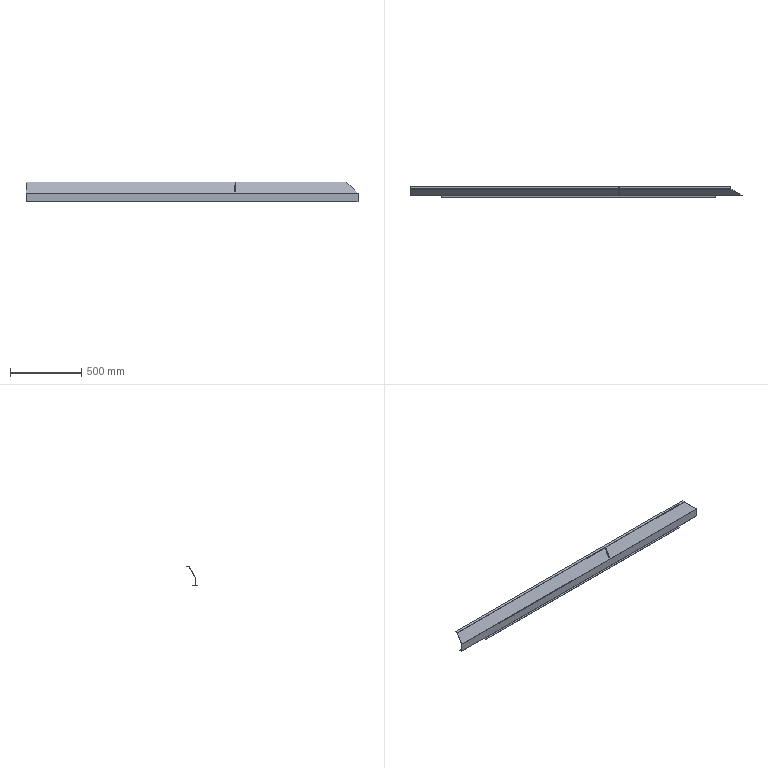Part | STEP file | Front Base Frame | 1 solid | 45 faces | box 2334 x 83.033 x 138 mm | volume 848369 mm3 | plane 31 | cylinder 14 | commonest cylinder face diameters 1 x9 5 x5
STEP:
#1=CARTESIAN_POINT('',(2150.,0.,-56.5));
#2=VERTEX_POINT('',#1);
#3=CARTESIAN_POINT('',(2149.5,0.,-56.));
#4=VERTEX_POINT('',#3);
#5=CARTESIAN_POINT('',(2149.5,0.,-56.5));
#6=DIRECTION('',(0.,-1.,0.));
#7=DIRECTION('',(0.,0.,1.));
#8=AXIS2_PLACEMENT_3D('',#5,#6,#7);
#9=CIRCLE('',#8,0.5);
#10=EDGE_CURVE('',#2,#4,#9,.T.);
#11=ORIENTED_EDGE('',*,*,#10,.T.);
#12=CARTESIAN_POINT('',(2149.5,2.,-56.));
#13=VERTEX_POINT('',#12);
#14=CARTESIAN_POINT('',(2149.5,0.,-56.));
#15=DIRECTION('',(0.,1.,0.));
#16=VECTOR('',#15,1000.);
#17=LINE('',#14,#16);
#18=EDGE_CURVE('',#4,#13,#17,.T.);
#19=ORIENTED_EDGE('',*,*,#18,.T.);
#20=CARTESIAN_POINT('',(2150.,2.,-56.5));
#21=VERTEX_POINT('',#20);
#22=CARTESIAN_POINT('',(2149.5,2.,-56.5));
#23=DIRECTION('',(0.,-1.,0.));
#24=DIRECTION('',(0.,0.,1.));
#25=AXIS2_PLACEMENT_3D('',#22,#23,#24);
#26=CIRCLE('',#25,0.5);
#27=EDGE_CURVE('',#21,#13,#26,.T.);
#28=ORIENTED_EDGE('',*,*,#27,.F.);
#29=CARTESIAN_POINT('',(2150.,0.,-56.5));
#30=DIRECTION('',(0.,1.,0.));
#31=VECTOR('',#30,1000.);
#32=LINE('',#29,#31);
#33=EDGE_CURVE('',#2,#21,#32,.T.);
#34=ORIENTED_EDGE('',*,*,#33,.F.);
#35=EDGE_LOOP('',(#11,#19,#28,#34));
#36=FACE_OUTER_BOUND('',#35,.T.);
#37=CARTESIAN_POINT('',(2149.5,0.,-56.5));
#38=DIRECTION('',(0.,1.,0.));
#39=DIRECTION('',(0.,0.,1.));
#40=AXIS2_PLACEMENT_3D('',#37,#38,#39);
#41=CYLINDRICAL_SURFACE('',#40,0.5);
#42=ADVANCED_FACE('',(#36),#41,.F.);
#43=CARTESIAN_POINT('',(219.5,0.,-56.));
#44=VERTEX_POINT('',#43);
#45=CARTESIAN_POINT('',(220.,0.,-56.5));
#46=VERTEX_POINT('',#45);
#47=CARTESIAN_POINT('',(219.5,0.,-56.5));
#48=DIRECTION('',(0.,1.,0.));
#49=DIRECTION('',(0.,0.,1.));
#50=AXIS2_PLACEMENT_3D('',#47,#48,#49);
#51=CIRCLE('',#50,0.5);
#52=EDGE_CURVE('',#44,#46,#51,.T.);
#53=ORIENTED_EDGE('',*,*,#52,.F.);
#54=CARTESIAN_POINT('',(219.5,2.,-56.));
#55=VERTEX_POINT('',#54);
#56=CARTESIAN_POINT('',(219.5,0.,-56.));
#57=DIRECTION('',(0.,1.,0.));
#58=VECTOR('',#57,1000.);
#59=LINE('',#56,#58);
#60=EDGE_CURVE('',#44,#55,#59,.T.);
#61=ORIENTED_EDGE('',*,*,#60,.T.);
#62=CARTESIAN_POINT('',(220.,2.,-56.5));
#63=VERTEX_POINT('',#62);
#64=CARTESIAN_POINT('',(219.5,2.,-56.5));
#65=DIRECTION('',(0.,-1.,0.));
#66=DIRECTION('',(0.,0.,1.));
#67=AXIS2_PLACEMENT_3D('',#64,#65,#66);
#68=CIRCLE('',#67,0.5);
#69=EDGE_CURVE('',#63,#55,#68,.T.);
#70=ORIENTED_EDGE('',*,*,#69,.F.);
#71=CARTESIAN_POINT('',(220.,0.,-56.5));
#72=DIRECTION('',(0.,1.,0.));
#73=VECTOR('',#72,1000.);
#74=LINE('',#71,#73);
#75=EDGE_CURVE('',#46,#63,#74,.T.);
#76=ORIENTED_EDGE('',*,*,#75,.F.);
#77=EDGE_LOOP('',(#53,#61,#70,#76));
#78=FACE_OUTER_BOUND('',#77,.T.);
#79=CARTESIAN_POINT('',(219.5,0.,-56.5));
#80=DIRECTION('',(0.,1.,0.));
#81=DIRECTION('',(0.,0.,1.));
#82=AXIS2_PLACEMENT_3D('',#79,#80,#81);
#83=CYLINDRICAL_SURFACE('',#82,0.5);
#84=ADVANCED_FACE('',(#78),#83,.F.);
#85=CARTESIAN_POINT('',(0.,2.067,-0.4199));
#86=VERTEX_POINT('',#85);
#87=CARTESIAN_POINT('',(0.,46.044,75.75));
#88=VERTEX_POINT('',#87);
#89=CARTESIAN_POINT('',(0.,46.765,77.));
#90=DIRECTION('',(0.,0.5,0.866));
#91=VECTOR('',#90,1000.);
#92=LINE('',#89,#91);
#93=EDGE_CURVE('',#86,#88,#92,.T.);
#94=ORIENTED_EDGE('',*,*,#93,.T.);
#95=CARTESIAN_POINT('',(1468.,46.044,75.75));
#96=VERTEX_POINT('',#95);
#97=CARTESIAN_POINT('',(2334.,46.044,75.75));
#98=DIRECTION('',(1.,0.,0.));
#99=VECTOR('',#98,1000.);
#100=LINE('',#97,#99);
#101=EDGE_CURVE('',#88,#96,#100,.T.);
#102=ORIENTED_EDGE('',*,*,#101,.T.);
#103=CARTESIAN_POINT('',(1468.,9.238,12.));
#104=VERTEX_POINT('',#103);
#105=CARTESIAN_POINT('',(1468.,46.765,77.));
#106=DIRECTION('',(0.,-0.5,-0.866));
#107=VECTOR('',#106,1000.);
#108=LINE('',#105,#107);
#109=EDGE_CURVE('',#96,#104,#108,.T.);
#110=ORIENTED_EDGE('',*,*,#109,.T.);
#111=CARTESIAN_POINT('',(1473.,9.238,12.));
#112=VERTEX_POINT('',#111);
#113=CARTESIAN_POINT('',(2334.,9.238,12.));
#114=DIRECTION('',(1.,0.,0.));
#115=VECTOR('',#114,1000.);
#116=LINE('',#113,#115);
#117=EDGE_CURVE('',#104,#112,#116,.T.);
#118=ORIENTED_EDGE('',*,*,#117,.T.);
#119=CARTESIAN_POINT('',(1473.,46.044,75.75));
#120=VERTEX_POINT('',#119);
#121=CARTESIAN_POINT('',(1473.,46.765,77.));
#122=DIRECTION('',(0.,0.5,0.866));
#123=VECTOR('',#122,1000.);
#124=LINE('',#121,#123);
#125=EDGE_CURVE('',#112,#120,#124,.T.);
#126=ORIENTED_EDGE('',*,*,#125,.T.);
#127=CARTESIAN_POINT('',(2255.,46.044,75.75));
#128=VERTEX_POINT('',#127);
#129=CARTESIAN_POINT('',(2334.,46.044,75.75));
#130=DIRECTION('',(1.,0.,0.));
#131=VECTOR('',#130,1000.);
#132=LINE('',#129,#131);
#133=EDGE_CURVE('',#120,#128,#132,.T.);
#134=ORIENTED_EDGE('',*,*,#133,.T.);
#135=CARTESIAN_POINT('',(2255.,46.032,75.73));
#136=VERTEX_POINT('',#135);
#137=CARTESIAN_POINT('',(2255.,46.044,75.75));
#138=DIRECTION('',(0.,-0.5,-0.866));
#139=VECTOR('',#138,1000.);
#140=LINE('',#137,#139);
#141=EDGE_CURVE('',#128,#136,#140,.T.);
#142=ORIENTED_EDGE('',*,*,#141,.T.);
#143=CARTESIAN_POINT('',(2333.105,2.067,-0.4199));
#144=VERTEX_POINT('',#143);
#145=CARTESIAN_POINT('',(2255.,46.032,75.73));
#146=DIRECTION('',(0.6641,-0.3738,-0.6475));
#147=VECTOR('',#146,1000.);
#148=LINE('',#145,#147);
#149=EDGE_CURVE('',#136,#144,#148,.T.);
#150=ORIENTED_EDGE('',*,*,#149,.T.);
#151=CARTESIAN_POINT('',(2334.,2.067,-0.4199));
#152=DIRECTION('',(-1.,0.,0.));
#153=VECTOR('',#152,1000.);
#154=LINE('',#151,#153);
#155=EDGE_CURVE('',#144,#86,#154,.T.);
#156=ORIENTED_EDGE('',*,*,#155,.T.);
#157=EDGE_LOOP('',(#94,#102,#110,#118,#126,#134,#142,#150,#156));
#158=FACE_OUTER_BOUND('',#157,.T.);
#159=CARTESIAN_POINT('',(2334.,46.765,77.));
#160=DIRECTION('',(0.,0.866,-0.5));
#161=DIRECTION('',(0.,0.5,0.866));
#162=AXIS2_PLACEMENT_3D('',#159,#160,#161);
#163=PLANE('',#162);
#164=ADVANCED_FACE('',(#158),#163,.T.);
#165=ORIENTED_EDGE('',*,*,#101,.F.);
#166=CARTESIAN_POINT('',(0.,46.477,76.));
#167=VERTEX_POINT('',#166);
#168=CARTESIAN_POINT('',(0.,46.477,75.5));
#169=DIRECTION('',(1.,0.,0.));
#170=DIRECTION('',(0.,0.,1.));
#171=AXIS2_PLACEMENT_3D('',#168,#169,#170);
#172=CIRCLE('',#171,0.5);
#173=EDGE_CURVE('',#167,#88,#172,.T.);
#174=ORIENTED_EDGE('',*,*,#173,.F.);
#175=CARTESIAN_POINT('',(1466.,46.477,76.));
#176=VERTEX_POINT('',#175);
#177=CARTESIAN_POINT('',(2334.,46.477,76.));
#178=DIRECTION('',(-1.,0.,0.));
#179=VECTOR('',#178,1000.);
#180=LINE('',#177,#179);
#181=EDGE_CURVE('',#176,#167,#180,.T.);
#182=ORIENTED_EDGE('',*,*,#181,.F.);
#183=CARTESIAN_POINT('',(1468.,46.477,76.));
#184=VERTEX_POINT('',#183);
#185=CARTESIAN_POINT('',(2334.,46.477,76.));
#186=DIRECTION('',(-1.,0.,0.));
#187=VECTOR('',#186,1000.);
#188=LINE('',#185,#187);
#189=EDGE_CURVE('',#184,#176,#188,.T.);
#190=ORIENTED_EDGE('',*,*,#189,.F.);
#191=CARTESIAN_POINT('',(1468.,46.477,75.5));
#192=DIRECTION('',(-1.,0.,0.));
#193=DIRECTION('',(0.,0.,1.));
#194=AXIS2_PLACEMENT_3D('',#191,#192,#193);
#195=CIRCLE('',#194,0.5);
#196=EDGE_CURVE('',#96,#184,#195,.T.);
#197=ORIENTED_EDGE('',*,*,#196,.F.);
#198=EDGE_LOOP('',(#165,#174,#182,#190,#197));
#199=FACE_OUTER_BOUND('',#198,.T.);
#200=CARTESIAN_POINT('',(2334.,46.477,75.5));
#201=DIRECTION('',(-1.,0.,0.));
#202=DIRECTION('',(0.,0.,1.));
#203=AXIS2_PLACEMENT_3D('',#200,#201,#202);
#204=CYLINDRICAL_SURFACE('',#203,0.5);
#205=ADVANCED_FACE('',(#199),#204,.F.);
#206=ORIENTED_EDGE('',*,*,#93,.F.);
#207=CARTESIAN_POINT('',(0.,2.,-0.6699));
#208=VERTEX_POINT('',#207);
#209=CARTESIAN_POINT('',(0.,2.5,-0.6699));
#210=DIRECTION('',(1.,0.,0.));
#211=DIRECTION('',(0.,0.,1.));
#212=AXIS2_PLACEMENT_3D('',#209,#210,#211);
#213=CIRCLE('',#212,0.5);
#214=EDGE_CURVE('',#86,#208,#213,.T.);
#215=ORIENTED_EDGE('',*,*,#214,.T.);
#216=CARTESIAN_POINT('',(0.,2.,-57.5));
#217=VERTEX_POINT('',#216);
#218=CARTESIAN_POINT('',(0.,2.,0.));
#219=DIRECTION('',(0.,0.,1.));
#220=VECTOR('',#219,1000.);
#221=LINE('',#218,#220);
#222=EDGE_CURVE('',#217,#208,#221,.T.);
#223=ORIENTED_EDGE('',*,*,#222,.F.);
#224=CARTESIAN_POINT('',(0.,2.5,-58.));
#225=VERTEX_POINT('',#224);
#226=CARTESIAN_POINT('',(0.,2.5,-57.5));
#227=DIRECTION('',(1.,0.,0.));
#228=DIRECTION('',(0.,0.,1.));
#229=AXIS2_PLACEMENT_3D('',#226,#227,#228);
#230=CIRCLE('',#229,0.5);
#231=EDGE_CURVE('',#217,#225,#230,.T.);
#232=ORIENTED_EDGE('',*,*,#231,.T.);
#233=CARTESIAN_POINT('',(0.,20.,-58.));
#234=VERTEX_POINT('',#233);
#235=CARTESIAN_POINT('',(0.,0.,-58.));
#236=DIRECTION('',(0.,1.,0.));
#237=VECTOR('',#236,1000.);
#238=LINE('',#235,#237);
#239=EDGE_CURVE('',#225,#234,#238,.T.);
#240=ORIENTED_EDGE('',*,*,#239,.T.);
#241=CARTESIAN_POINT('',(0.,20.,-60.));
#242=VERTEX_POINT('',#241);
#243=CARTESIAN_POINT('',(0.,20.,-60.));
#244=DIRECTION('',(0.,0.,-1.));
#245=VECTOR('',#244,1000.);
#246=LINE('',#243,#245);
#247=EDGE_CURVE('',#234,#242,#246,.T.);
#248=ORIENTED_EDGE('',*,*,#247,.T.);
#249=CARTESIAN_POINT('',(0.,2.5,-60.));
#250=VERTEX_POINT('',#249);
#251=CARTESIAN_POINT('',(0.,2.,-60.));
#252=DIRECTION('',(0.,-1.,0.));
#253=VECTOR('',#252,1000.);
#254=LINE('',#251,#253);
#255=EDGE_CURVE('',#242,#250,#254,.T.);
#256=ORIENTED_EDGE('',*,*,#255,.T.);
#257=CARTESIAN_POINT('',(0.,0.,-57.5));
#258=VERTEX_POINT('',#257);
#259=CARTESIAN_POINT('',(0.,2.5,-57.5));
#260=DIRECTION('',(1.,0.,0.));
#261=DIRECTION('',(0.,0.,1.));
#262=AXIS2_PLACEMENT_3D('',#259,#260,#261);
#263=CIRCLE('',#262,2.5);
#264=EDGE_CURVE('',#258,#250,#263,.T.);
#265=ORIENTED_EDGE('',*,*,#264,.F.);
#266=CARTESIAN_POINT('',(0.,0.,-0.6699));
#267=VERTEX_POINT('',#266);
#268=CARTESIAN_POINT('',(0.,0.,-0.4199));
#269=DIRECTION('',(0.,0.,1.));
#270=VECTOR('',#269,1000.);
#271=LINE('',#268,#270);
#272=EDGE_CURVE('',#258,#267,#271,.T.);
#273=ORIENTED_EDGE('',*,*,#272,.T.);
#274=CARTESIAN_POINT('',(0.,0.3349,0.5801));
#275=VERTEX_POINT('',#274);
#276=CARTESIAN_POINT('',(0.,2.5,-0.6699));
#277=DIRECTION('',(-1.,0.,0.));
#278=DIRECTION('',(0.,0.,1.));
#279=AXIS2_PLACEMENT_3D('',#276,#277,#278);
#280=CIRCLE('',#279,2.5);
#281=EDGE_CURVE('',#267,#275,#280,.T.);
#282=ORIENTED_EDGE('',*,*,#281,.T.);
#283=CARTESIAN_POINT('',(0.,44.312,76.75));
#284=VERTEX_POINT('',#283);
#285=CARTESIAN_POINT('',(0.,0.3349,0.5801));
#286=DIRECTION('',(0.,0.5,0.866));
#287=VECTOR('',#286,1000.);
#288=LINE('',#285,#287);
#289=EDGE_CURVE('',#275,#284,#288,.T.);
#290=ORIENTED_EDGE('',*,*,#289,.T.);
#291=CARTESIAN_POINT('',(0.,46.477,78.));
#292=VERTEX_POINT('',#291);
#293=CARTESIAN_POINT('',(0.,46.477,75.5));
#294=DIRECTION('',(-1.,0.,0.));
#295=DIRECTION('',(0.,0.,1.));
#296=AXIS2_PLACEMENT_3D('',#293,#294,#295);
#297=CIRCLE('',#296,2.5);
#298=EDGE_CURVE('',#284,#292,#297,.T.);
#299=ORIENTED_EDGE('',*,*,#298,.T.);
#300=CARTESIAN_POINT('',(0.,65.033,78.));
#301=VERTEX_POINT('',#300);
#302=CARTESIAN_POINT('',(0.,2.5,78.));
#303=DIRECTION('',(0.,-1.,0.));
#304=VECTOR('',#303,1000.);
#305=LINE('',#302,#304);
#306=EDGE_CURVE('',#301,#292,#305,.T.);
#307=ORIENTED_EDGE('',*,*,#306,.F.);
#308=CARTESIAN_POINT('',(0.,65.033,76.));
#309=VERTEX_POINT('',#308);
#310=CARTESIAN_POINT('',(0.,65.033,78.));
#311=DIRECTION('',(0.,0.,1.));
#312=VECTOR('',#311,1000.);
#313=LINE('',#310,#312);
#314=EDGE_CURVE('',#309,#301,#313,.T.);
#315=ORIENTED_EDGE('',*,*,#314,.F.);
#316=CARTESIAN_POINT('',(0.,65.033,76.));
#317=DIRECTION('',(0.,1.,0.));
#318=VECTOR('',#317,1000.);
#319=LINE('',#316,#318);
#320=EDGE_CURVE('',#167,#309,#319,.T.);
#321=ORIENTED_EDGE('',*,*,#320,.F.);
#322=ORIENTED_EDGE('',*,*,#173,.T.);
#323=EDGE_LOOP('',(#206,#215,#223,#232,#240,#248,#256,#265,#273,#282,#290,#299,#307,#315,#321,#322));
#324=FACE_OUTER_BOUND('',#323,.T.);
#325=CARTESIAN_POINT('',(0.,46.477,76.));
#326=DIRECTION('',(-1.,0.,0.));
#327=DIRECTION('',(0.,0.,1.));
#328=AXIS2_PLACEMENT_3D('',#325,#326,#327);
#329=PLANE('',#328);
#330=ADVANCED_FACE('',(#324),#329,.T.);
#331=CARTESIAN_POINT('',(2333.361,2.,-0.6699));
#332=VERTEX_POINT('',#331);
#333=CARTESIAN_POINT('',(2334.,2.,-0.6699));
#334=DIRECTION('',(1.,0.,0.));
#335=VECTOR('',#334,1000.);
#336=LINE('',#333,#335);
#337=EDGE_CURVE('',#208,#332,#336,.T.);
#338=ORIENTED_EDGE('',*,*,#337,.F.);
#339=ORIENTED_EDGE('',*,*,#214,.F.);
#340=ORIENTED_EDGE('',*,*,#155,.F.);
#341=CARTESIAN_POINT('',(2333.361,2.,-0.6699));
#342=CARTESIAN_POINT('',(2333.271,2.,-0.5816));
#343=CARTESIAN_POINT('',(2333.183,2.023,-0.4963));
#344=CARTESIAN_POINT('',(2333.105,2.067,-0.4199));
#345=(BOUNDED_CURVE()B_SPLINE_CURVE(3,(#341,#342,#343,#344),.UNSPECIFIED.,.F.,.F.)B_SPLINE_CURVE_WITH_KNOTS((4,4),(4.712,5.236),.UNSPECIFIED.)CURVE()GEOMETRIC_REPRESENTATION_ITEM()RATIONAL_B_SPLINE_CURVE((1.,0.9773,0.9773,1.))REPRESENTATION_ITEM(''));
#346=EDGE_CURVE('',#332,#144,#345,.T.);
#347=ORIENTED_EDGE('',*,*,#346,.F.);
#348=EDGE_LOOP('',(#338,#339,#340,#347));
#349=FACE_OUTER_BOUND('',#348,.T.);
#350=CARTESIAN_POINT('',(2334.,2.5,-0.6699));
#351=DIRECTION('',(-1.,0.,0.));
#352=DIRECTION('',(0.,0.,1.));
#353=AXIS2_PLACEMENT_3D('',#350,#351,#352);
#354=CYLINDRICAL_SURFACE('',#353,0.5);
#355=ADVANCED_FACE('',(#349),#354,.F.);
#356=ORIENTED_EDGE('',*,*,#346,.T.);
#357=ORIENTED_EDGE('',*,*,#149,.F.);
#358=CARTESIAN_POINT('',(2255.,43.723,75.73));
#359=VERTEX_POINT('',#358);
#360=CARTESIAN_POINT('',(2255.,-18.,75.73));
#361=DIRECTION('',(0.,1.,0.));
#362=VECTOR('',#361,1000.);
#363=LINE('',#360,#362);
#364=EDGE_CURVE('',#359,#136,#363,.T.);
#365=ORIENTED_EDGE('',*,*,#364,.F.);
#366=CARTESIAN_POINT('',(2332.079,0.3349,0.5801));
#367=VERTEX_POINT('',#366);
#368=CARTESIAN_POINT('',(2332.079,0.3349,0.5801));
#369=DIRECTION('',(-0.6641,0.3738,0.6475));
#370=VECTOR('',#369,1000.);
#371=LINE('',#368,#370);
#372=EDGE_CURVE('',#367,#359,#371,.T.);
#373=ORIENTED_EDGE('',*,*,#372,.F.);
#374=CARTESIAN_POINT('',(2333.361,0.,-0.6699));
#375=VERTEX_POINT('',#374);
#376=CARTESIAN_POINT('',(2333.361,0.,-0.6699));
#377=CARTESIAN_POINT('',(2332.909,0.,-0.2285));
#378=CARTESIAN_POINT('',(2332.471,0.1142,0.1979));
#379=CARTESIAN_POINT('',(2332.079,0.3349,0.5801));
#380=(BOUNDED_CURVE()B_SPLINE_CURVE(3,(#376,#377,#378,#379),.UNSPECIFIED.,.F.,.F.)B_SPLINE_CURVE_WITH_KNOTS((4,4),(4.712,5.236),.UNSPECIFIED.)CURVE()GEOMETRIC_REPRESENTATION_ITEM()RATIONAL_B_SPLINE_CURVE((1.,0.9773,0.9773,1.))REPRESENTATION_ITEM(''));
#381=EDGE_CURVE('',#375,#367,#380,.T.);
#382=ORIENTED_EDGE('',*,*,#381,.F.);
#383=CARTESIAN_POINT('',(2333.7,0.,-1.));
#384=VERTEX_POINT('',#383);
#385=CARTESIAN_POINT('',(2333.361,0.,-0.6699));
#386=DIRECTION('',(0.716,0.,-0.6981));
#387=VECTOR('',#386,1000.);
#388=LINE('',#385,#387);
#389=EDGE_CURVE('',#375,#384,#388,.T.);
#390=ORIENTED_EDGE('',*,*,#389,.T.);
#391=CARTESIAN_POINT('',(2333.7,2.,-1.));
#392=VERTEX_POINT('',#391);
#393=CARTESIAN_POINT('',(2333.7,-18.,-1.));
#394=DIRECTION('',(0.,-1.,0.));
#395=VECTOR('',#394,1000.);
#396=LINE('',#393,#395);
#397=EDGE_CURVE('',#392,#384,#396,.T.);
#398=ORIENTED_EDGE('',*,*,#397,.F.);
#399=CARTESIAN_POINT('',(2255.,2.,75.73));
#400=DIRECTION('',(0.716,0.,-0.6981));
#401=VECTOR('',#400,1000.);
#402=LINE('',#399,#401);
#403=EDGE_CURVE('',#332,#392,#402,.T.);
#404=ORIENTED_EDGE('',*,*,#403,.F.);
#405=EDGE_LOOP('',(#356,#357,#365,#373,#382,#390,#398,#404));
#406=FACE_OUTER_BOUND('',#405,.T.);
#407=CARTESIAN_POINT('',(2255.,-18.,75.73));
#408=DIRECTION('',(-0.6981,0.,-0.716));
#409=DIRECTION('',(-0.716,0.,0.6981));
#410=AXIS2_PLACEMENT_3D('',#407,#408,#409);
#411=PLANE('',#410);
#412=ADVANCED_FACE('',(#406),#411,.F.);
#413=CARTESIAN_POINT('',(2255.,46.477,76.));
#414=VERTEX_POINT('',#413);
#415=CARTESIAN_POINT('',(1473.,46.477,76.));
#416=VERTEX_POINT('',#415);
#417=CARTESIAN_POINT('',(2334.,46.477,76.));
#418=DIRECTION('',(-1.,0.,0.));
#419=VECTOR('',#418,1000.);
#420=LINE('',#417,#419);
#421=EDGE_CURVE('',#414,#416,#420,.T.);
#422=ORIENTED_EDGE('',*,*,#421,.F.);
#423=CARTESIAN_POINT('',(2255.,46.477,75.5));
#424=DIRECTION('',(-1.,0.,0.));
#425=DIRECTION('',(0.,0.,1.));
#426=AXIS2_PLACEMENT_3D('',#423,#424,#425);
#427=CIRCLE('',#426,0.5);
#428=EDGE_CURVE('',#128,#414,#427,.T.);
#429=ORIENTED_EDGE('',*,*,#428,.F.);
#430=ORIENTED_EDGE('',*,*,#133,.F.);
#431=CARTESIAN_POINT('',(1473.,46.477,75.5));
#432=DIRECTION('',(1.,0.,0.));
#433=DIRECTION('',(0.,0.,1.));
#434=AXIS2_PLACEMENT_3D('',#431,#432,#433);
#435=CIRCLE('',#434,0.5);
#436=EDGE_CURVE('',#416,#120,#435,.T.);
#437=ORIENTED_EDGE('',*,*,#436,.F.);
#438=EDGE_LOOP('',(#422,#429,#430,#437));
#439=FACE_OUTER_BOUND('',#438,.T.);
#440=CARTESIAN_POINT('',(2334.,46.477,75.5));
#441=DIRECTION('',(-1.,0.,0.));
#442=DIRECTION('',(0.,0.,1.));
#443=AXIS2_PLACEMENT_3D('',#440,#441,#442);
#444=CYLINDRICAL_SURFACE('',#443,0.5);
#445=ADVANCED_FACE('',(#439),#444,.F.);
#446=ORIENTED_EDGE('',*,*,#436,.T.);
#447=ORIENTED_EDGE('',*,*,#125,.F.);
#448=CARTESIAN_POINT('',(1473.,6.928,12.));
#449=VERTEX_POINT('',#448);
#450=CARTESIAN_POINT('',(1473.,-18.,12.));
#451=DIRECTION('',(0.,1.,0.));
#452=VECTOR('',#451,1000.);
#453=LINE('',#450,#452);
#454=EDGE_CURVE('',#449,#112,#453,.T.);
#455=ORIENTED_EDGE('',*,*,#454,.F.);
#456=CARTESIAN_POINT('',(1473.,44.312,76.75));
#457=VERTEX_POINT('',#456);
#458=CARTESIAN_POINT('',(1473.,44.312,76.75));
#459=DIRECTION('',(0.,-0.5,-0.866));
#460=VECTOR('',#459,1000.);
#461=LINE('',#458,#460);
#462=EDGE_CURVE('',#457,#449,#461,.T.);
#463=ORIENTED_EDGE('',*,*,#462,.F.);
#464=CARTESIAN_POINT('',(1473.,46.477,78.));
#465=VERTEX_POINT('',#464);
#466=CARTESIAN_POINT('',(1473.,46.477,75.5));
#467=DIRECTION('',(1.,0.,0.));
#468=DIRECTION('',(0.,0.,1.));
#469=AXIS2_PLACEMENT_3D('',#466,#467,#468);
#470=CIRCLE('',#469,2.5);
#471=EDGE_CURVE('',#465,#457,#470,.T.);
#472=ORIENTED_EDGE('',*,*,#471,.F.);
#473=CARTESIAN_POINT('',(1473.,65.033,78.));
#474=VERTEX_POINT('',#473);
#475=CARTESIAN_POINT('',(1473.,-18.,78.));
#476=DIRECTION('',(0.,-1.,0.));
#477=VECTOR('',#476,1000.);
#478=LINE('',#475,#477);
#479=EDGE_CURVE('',#474,#465,#478,.T.);
#480=ORIENTED_EDGE('',*,*,#479,.F.);
#481=CARTESIAN_POINT('',(1473.,65.033,76.));
#482=VERTEX_POINT('',#481);
#483=CARTESIAN_POINT('',(1473.,65.033,78.));
#484=DIRECTION('',(0.,0.,1.));
#485=VECTOR('',#484,1000.);
#486=LINE('',#483,#485);
#487=EDGE_CURVE('',#482,#474,#486,.T.);
#488=ORIENTED_EDGE('',*,*,#487,.F.);
#489=CARTESIAN_POINT('',(1473.,-18.,76.));
#490=DIRECTION('',(0.,1.,0.));
#491=VECTOR('',#490,1000.);
#492=LINE('',#489,#491);
#493=EDGE_CURVE('',#416,#482,#492,.T.);
#494=ORIENTED_EDGE('',*,*,#493,.F.);
#495=EDGE_LOOP('',(#446,#447,#455,#463,#472,#480,#488,#494));
#496=FACE_OUTER_BOUND('',#495,.T.);
#497=CARTESIAN_POINT('',(1473.,-18.,78.));
#498=DIRECTION('',(1.,0.,0.));
#499=DIRECTION('',(0.,0.,-1.));
#500=AXIS2_PLACEMENT_3D('',#497,#498,#499);
#501=PLANE('',#500);
#502=ADVANCED_FACE('',(#496),#501,.F.);
#503=CARTESIAN_POINT('',(1468.,6.928,12.));
#504=VERTEX_POINT('',#503);
#505=CARTESIAN_POINT('',(1468.,-18.,12.));
#506=DIRECTION('',(0.,1.,0.));
#507=VECTOR('',#506,1000.);
#508=LINE('',#505,#507);
#509=EDGE_CURVE('',#504,#104,#508,.T.);
#510=ORIENTED_EDGE('',*,*,#509,.F.);
#511=CARTESIAN_POINT('',(1468.,6.928,12.));
#512=DIRECTION('',(-1.,0.,0.));
#513=VECTOR('',#512,1000.);
#514=LINE('',#511,#513);
#515=EDGE_CURVE('',#449,#504,#514,.T.);
#516=ORIENTED_EDGE('',*,*,#515,.F.);
#517=ORIENTED_EDGE('',*,*,#454,.T.);
#518=ORIENTED_EDGE('',*,*,#117,.F.);
#519=EDGE_LOOP('',(#510,#516,#517,#518));
#520=FACE_OUTER_BOUND('',#519,.T.);
#521=CARTESIAN_POINT('',(1468.,-18.,12.));
#522=DIRECTION('',(0.,0.,-1.));
#523=DIRECTION('',(0.,1.,0.));
#524=AXIS2_PLACEMENT_3D('',#521,#522,#523);
#525=PLANE('',#524);
#526=ADVANCED_FACE('',(#520),#525,.F.);
#527=ORIENTED_EDGE('',*,*,#109,.F.);
#528=ORIENTED_EDGE('',*,*,#196,.T.);
#529=CARTESIAN_POINT('',(1468.,46.477,78.));
#530=VERTEX_POINT('',#529);
#531=CARTESIAN_POINT('',(1468.,46.477,78.));
#532=DIRECTION('',(0.,0.,-1.));
#533=VECTOR('',#532,1000.);
#534=LINE('',#531,#533);
#535=EDGE_CURVE('',#530,#184,#534,.T.);
#536=ORIENTED_EDGE('',*,*,#535,.F.);
#537=CARTESIAN_POINT('',(1468.,44.312,76.75));
#538=VERTEX_POINT('',#537);
#539=CARTESIAN_POINT('',(1468.,46.477,75.5));
#540=DIRECTION('',(-1.,0.,0.));
#541=DIRECTION('',(0.,0.,1.));
#542=AXIS2_PLACEMENT_3D('',#539,#540,#541);
#543=CIRCLE('',#542,2.5);
#544=EDGE_CURVE('',#538,#530,#543,.T.);
#545=ORIENTED_EDGE('',*,*,#544,.F.);
#546=CARTESIAN_POINT('',(1468.,6.928,12.));
#547=DIRECTION('',(0.,0.5,0.866));
#548=VECTOR('',#547,1000.);
#549=LINE('',#546,#548);
#550=EDGE_CURVE('',#504,#538,#549,.T.);
#551=ORIENTED_EDGE('',*,*,#550,.F.);
#552=ORIENTED_EDGE('',*,*,#509,.T.);
#553=EDGE_LOOP('',(#527,#528,#536,#545,#551,#552));
#554=FACE_OUTER_BOUND('',#553,.T.);
#555=CARTESIAN_POINT('',(1468.,-18.,78.));
#556=DIRECTION('',(-1.,0.,0.));
#557=DIRECTION('',(0.,0.,1.));
#558=AXIS2_PLACEMENT_3D('',#555,#556,#557);
#559=PLANE('',#558);
#560=ADVANCED_FACE('',(#554),#559,.F.);
#561=ORIENTED_EDGE('',*,*,#320,.T.);
#562=CARTESIAN_POINT('',(1466.,65.033,76.));
#563=VERTEX_POINT('',#562);
#564=CARTESIAN_POINT('',(2334.,65.033,76.));
#565=DIRECTION('',(1.,0.,0.));
#566=VECTOR('',#565,1000.);
#567=LINE('',#564,#566);
#568=EDGE_CURVE('',#309,#563,#567,.T.);
#569=ORIENTED_EDGE('',*,*,#568,.T.);
#570=CARTESIAN_POINT('',(1466.,65.033,76.));
#571=DIRECTION('',(0.,-1.,0.));
#572=VECTOR('',#571,1000.);
#573=LINE('',#570,#572);
#574=EDGE_CURVE('',#563,#176,#573,.T.);
#575=ORIENTED_EDGE('',*,*,#574,.T.);
#576=ORIENTED_EDGE('',*,*,#181,.T.);
#577=EDGE_LOOP('',(#561,#569,#575,#576));
#578=FACE_OUTER_BOUND('',#577,.T.);
#579=CARTESIAN_POINT('',(2334.,65.033,76.));
#580=DIRECTION('',(0.,0.,-1.));
#581=DIRECTION('',(0.,1.,0.));
#582=AXIS2_PLACEMENT_3D('',#579,#580,#581);
#583=PLANE('',#582);
#584=ADVANCED_FACE('',(#578),#583,.T.);
#585=ORIENTED_EDGE('',*,*,#535,.T.);
#586=ORIENTED_EDGE('',*,*,#189,.T.);
#587=CARTESIAN_POINT('',(1466.,46.477,78.));
#588=VERTEX_POINT('',#587);
#589=CARTESIAN_POINT('',(1466.,46.477,78.));
#590=DIRECTION('',(0.,0.,-1.));
#591=VECTOR('',#590,1000.);
#592=LINE('',#589,#591);
#593=EDGE_CURVE('',#588,#176,#592,.T.);
#594=ORIENTED_EDGE('',*,*,#593,.F.);
#595=CARTESIAN_POINT('',(1472.,46.477,78.));
#596=DIRECTION('',(-1.,0.,0.));
#597=VECTOR('',#596,1000.);
#598=LINE('',#595,#597);
#599=EDGE_CURVE('',#530,#588,#598,.T.);
#600=ORIENTED_EDGE('',*,*,#599,.F.);
#601=EDGE_LOOP('',(#585,#586,#594,#600));
#602=FACE_OUTER_BOUND('',#601,.T.);
#603=CARTESIAN_POINT('',(1472.,46.477,78.));
#604=DIRECTION('',(0.,-1.,0.));
#605=DIRECTION('',(0.,0.,-1.));
#606=AXIS2_PLACEMENT_3D('',#603,#604,#605);
#607=PLANE('',#606);
#608=ADVANCED_FACE('',(#602),#607,.F.);
#609=ORIENTED_EDGE('',*,*,#550,.T.);
#610=CARTESIAN_POINT('',(2334.,44.312,76.75));
#611=DIRECTION('',(1.,0.,0.));
#612=VECTOR('',#611,1000.);
#613=LINE('',#610,#612);
#614=EDGE_CURVE('',#284,#538,#613,.T.);
#615=ORIENTED_EDGE('',*,*,#614,.F.);
#616=ORIENTED_EDGE('',*,*,#289,.F.);
#617=CARTESIAN_POINT('',(2334.,0.3349,0.5801));
#618=DIRECTION('',(-1.,0.,0.));
#619=VECTOR('',#618,1000.);
#620=LINE('',#617,#619);
#621=EDGE_CURVE('',#367,#275,#620,.T.);
#622=ORIENTED_EDGE('',*,*,#621,.F.);
#623=ORIENTED_EDGE('',*,*,#372,.T.);
#624=CARTESIAN_POINT('',(2255.,44.312,76.75));
#625=VERTEX_POINT('',#624);
#626=CARTESIAN_POINT('',(2255.,45.033,78.));
#627=DIRECTION('',(0.,-0.5,-0.866));
#628=VECTOR('',#627,1000.);
#629=LINE('',#626,#628);
#630=EDGE_CURVE('',#625,#359,#629,.T.);
#631=ORIENTED_EDGE('',*,*,#630,.F.);
#632=CARTESIAN_POINT('',(2334.,44.312,76.75));
#633=DIRECTION('',(1.,0.,0.));
#634=VECTOR('',#633,1000.);
#635=LINE('',#632,#634);
#636=EDGE_CURVE('',#457,#625,#635,.T.);
#637=ORIENTED_EDGE('',*,*,#636,.F.);
#638=ORIENTED_EDGE('',*,*,#462,.T.);
#639=ORIENTED_EDGE('',*,*,#515,.T.);
#640=EDGE_LOOP('',(#609,#615,#616,#622,#623,#631,#637,#638,#639));
#641=FACE_OUTER_BOUND('',#640,.T.);
#642=CARTESIAN_POINT('',(2334.,45.033,78.));
#643=DIRECTION('',(0.,0.866,-0.5));
#644=DIRECTION('',(0.,0.5,0.866));
#645=AXIS2_PLACEMENT_3D('',#642,#643,#644);
#646=PLANE('',#645);
#647=ADVANCED_FACE('',(#641),#646,.F.);
#648=ORIENTED_EDGE('',*,*,#222,.T.);
#649=ORIENTED_EDGE('',*,*,#337,.T.);
#650=ORIENTED_EDGE('',*,*,#403,.T.);
#651=CARTESIAN_POINT('',(2334.,2.,-1.));
#652=VERTEX_POINT('',#651);
#653=CARTESIAN_POINT('',(2334.,2.,-1.));
#654=DIRECTION('',(1.,0.,0.));
#655=VECTOR('',#654,1000.);
#656=LINE('',#653,#655);
#657=EDGE_CURVE('',#392,#652,#656,.T.);
#658=ORIENTED_EDGE('',*,*,#657,.T.);
#659=CARTESIAN_POINT('',(2334.,2.,-60.));
#660=VERTEX_POINT('',#659);
#661=CARTESIAN_POINT('',(2334.,2.,0.));
#662=DIRECTION('',(0.,0.,-1.));
#663=VECTOR('',#662,1000.);
#664=LINE('',#661,#663);
#665=EDGE_CURVE('',#652,#660,#664,.T.);
#666=ORIENTED_EDGE('',*,*,#665,.T.);
#667=CARTESIAN_POINT('',(2150.,2.,-60.));
#668=VERTEX_POINT('',#667);
#669=CARTESIAN_POINT('',(2334.,2.,-60.));
#670=DIRECTION('',(-1.,0.,0.));
#671=VECTOR('',#670,1000.);
#672=LINE('',#669,#671);
#673=EDGE_CURVE('',#660,#668,#672,.T.);
#674=ORIENTED_EDGE('',*,*,#673,.T.);
#675=CARTESIAN_POINT('',(2150.,2.,0.));
#676=DIRECTION('',(0.,0.,1.));
#677=VECTOR('',#676,1000.);
#678=LINE('',#675,#677);
#679=EDGE_CURVE('',#668,#21,#678,.T.);
#680=ORIENTED_EDGE('',*,*,#679,.T.);
#681=ORIENTED_EDGE('',*,*,#27,.T.);
#682=CARTESIAN_POINT('',(2149.,2.,-56.5));
#683=VERTEX_POINT('',#682);
#684=CARTESIAN_POINT('',(2149.5,2.,-56.5));
#685=DIRECTION('',(0.,-1.,0.));
#686=DIRECTION('',(0.,0.,1.));
#687=AXIS2_PLACEMENT_3D('',#684,#685,#686);
#688=CIRCLE('',#687,0.5);
#689=EDGE_CURVE('',#13,#683,#688,.T.);
#690=ORIENTED_EDGE('',*,*,#689,.T.);
#691=CARTESIAN_POINT('',(2149.,2.,-57.5));
#692=VERTEX_POINT('',#691);
#693=CARTESIAN_POINT('',(2149.,2.,-56.5));
#694=DIRECTION('',(0.,0.,1.));
#695=VECTOR('',#694,1000.);
#696=LINE('',#693,#695);
#697=EDGE_CURVE('',#692,#683,#696,.T.);
#698=ORIENTED_EDGE('',*,*,#697,.F.);
#699=CARTESIAN_POINT('',(220.,2.,-57.5));
#700=VERTEX_POINT('',#699);
#701=CARTESIAN_POINT('',(2334.,2.,-57.5));
#702=DIRECTION('',(-1.,0.,0.));
#703=VECTOR('',#702,1000.);
#704=LINE('',#701,#703);
#705=EDGE_CURVE('',#692,#700,#704,.T.);
#706=ORIENTED_EDGE('',*,*,#705,.T.);
#707=CARTESIAN_POINT('',(220.,2.,-57.5));
#708=DIRECTION('',(0.,0.,-1.));
#709=VECTOR('',#708,1000.);
#710=LINE('',#707,#709);
#711=EDGE_CURVE('',#63,#700,#710,.T.);
#712=ORIENTED_EDGE('',*,*,#711,.F.);
#713=ORIENTED_EDGE('',*,*,#69,.T.);
#714=CARTESIAN_POINT('',(219.,2.,-56.5));
#715=VERTEX_POINT('',#714);
#716=CARTESIAN_POINT('',(219.5,2.,-56.5));
#717=DIRECTION('',(0.,-1.,0.));
#718=DIRECTION('',(0.,0.,1.));
#719=AXIS2_PLACEMENT_3D('',#716,#717,#718);
#720=CIRCLE('',#719,0.5);
#721=EDGE_CURVE('',#55,#715,#720,.T.);
#722=ORIENTED_EDGE('',*,*,#721,.T.);
#723=CARTESIAN_POINT('',(219.,2.,-57.5));
#724=VERTEX_POINT('',#723);
#725=CARTESIAN_POINT('',(219.,2.,-56.5));
#726=DIRECTION('',(0.,0.,1.));
#727=VECTOR('',#726,1000.);
#728=LINE('',#725,#727);
#729=EDGE_CURVE('',#724,#715,#728,.T.);
#730=ORIENTED_EDGE('',*,*,#729,.F.);
#731=CARTESIAN_POINT('',(2334.,2.,-57.5));
#732=DIRECTION('',(-1.,0.,0.));
#733=VECTOR('',#732,1000.);
#734=LINE('',#731,#733);
#735=EDGE_CURVE('',#724,#217,#734,.T.);
#736=ORIENTED_EDGE('',*,*,#735,.T.);
#737=EDGE_LOOP('',(#648,#649,#650,#658,#666,#674,#680,#681,#690,#698,#706,#712,#713,#722,#730,#736));
#738=FACE_OUTER_BOUND('',#737,.T.);
#739=CARTESIAN_POINT('',(2334.,2.,0.));
#740=DIRECTION('',(0.,1.,0.));
#741=DIRECTION('',(0.,0.,1.));
#742=AXIS2_PLACEMENT_3D('',#739,#740,#741);
#743=PLANE('',#742);
#744=ADVANCED_FACE('',(#738),#743,.T.);
#745=ORIENTED_EDGE('',*,*,#428,.T.);
#746=CARTESIAN_POINT('',(2255.,65.033,76.));
#747=VERTEX_POINT('',#746);
#748=CARTESIAN_POINT('',(2255.,-18.,76.));
#749=DIRECTION('',(0.,-1.,0.));
#750=VECTOR('',#749,1000.);
#751=LINE('',#748,#750);
#752=EDGE_CURVE('',#747,#414,#751,.T.);
#753=ORIENTED_EDGE('',*,*,#752,.F.);
#754=CARTESIAN_POINT('',(2255.,65.033,78.));
#755=VERTEX_POINT('',#754);
#756=CARTESIAN_POINT('',(2255.,65.033,75.73));
#757=DIRECTION('',(0.,0.,-1.));
#758=VECTOR('',#757,1000.);
#759=LINE('',#756,#758);
#760=EDGE_CURVE('',#755,#747,#759,.T.);
#761=ORIENTED_EDGE('',*,*,#760,.F.);
#762=CARTESIAN_POINT('',(2255.,46.477,78.));
#763=VERTEX_POINT('',#762);
#764=CARTESIAN_POINT('',(2255.,-18.,78.));
#765=DIRECTION('',(0.,1.,0.));
#766=VECTOR('',#765,1000.);
#767=LINE('',#764,#766);
#768=EDGE_CURVE('',#763,#755,#767,.T.);
#769=ORIENTED_EDGE('',*,*,#768,.F.);
#770=CARTESIAN_POINT('',(2255.,46.477,75.5));
#771=DIRECTION('',(-1.,0.,0.));
#772=DIRECTION('',(0.,0.,1.));
#773=AXIS2_PLACEMENT_3D('',#770,#771,#772);
#774=CIRCLE('',#773,2.5);
#775=EDGE_CURVE('',#625,#763,#774,.T.);
#776=ORIENTED_EDGE('',*,*,#775,.F.);
#777=ORIENTED_EDGE('',*,*,#630,.T.);
#778=ORIENTED_EDGE('',*,*,#364,.T.);
#779=ORIENTED_EDGE('',*,*,#141,.F.);
#780=EDGE_LOOP('',(#745,#753,#761,#769,#776,#777,#778,#779));
#781=FACE_OUTER_BOUND('',#780,.T.);
#782=CARTESIAN_POINT('',(2255.,-18.,75.73));
#783=DIRECTION('',(-1.,0.,0.));
#784=DIRECTION('',(0.,0.,1.));
#785=AXIS2_PLACEMENT_3D('',#782,#783,#784);
#786=PLANE('',#785);
#787=ADVANCED_FACE('',(#781),#786,.F.);
#788=ORIENTED_EDGE('',*,*,#621,.T.);
#789=ORIENTED_EDGE('',*,*,#281,.F.);
#790=CARTESIAN_POINT('',(2334.,0.,-0.6699));
#791=DIRECTION('',(1.,0.,0.));
#792=VECTOR('',#791,1000.);
#793=LINE('',#790,#792);
#794=EDGE_CURVE('',#267,#375,#793,.T.);
#795=ORIENTED_EDGE('',*,*,#794,.T.);
#796=ORIENTED_EDGE('',*,*,#381,.T.);
#797=EDGE_LOOP('',(#788,#789,#795,#796));
#798=FACE_OUTER_BOUND('',#797,.T.);
#799=CARTESIAN_POINT('',(2334.,2.5,-0.6699));
#800=DIRECTION('',(-1.,0.,0.));
#801=DIRECTION('',(0.,0.,1.));
#802=AXIS2_PLACEMENT_3D('',#799,#800,#801);
#803=CYLINDRICAL_SURFACE('',#802,2.5);
#804=ADVANCED_FACE('',(#798),#803,.T.);
#805=ORIENTED_EDGE('',*,*,#657,.F.);
#806=ORIENTED_EDGE('',*,*,#397,.T.);
#807=CARTESIAN_POINT('',(2334.,0.,-1.));
#808=VERTEX_POINT('',#807);
#809=CARTESIAN_POINT('',(2334.,0.,-1.));
#810=DIRECTION('',(-1.,0.,0.));
#811=VECTOR('',#810,1000.);
#812=LINE('',#809,#811);
#813=EDGE_CURVE('',#808,#384,#812,.T.);
#814=ORIENTED_EDGE('',*,*,#813,.F.);
#815=CARTESIAN_POINT('',(2334.,-18.,-1.));
#816=DIRECTION('',(0.,-1.,0.));
#817=VECTOR('',#816,1000.);
#818=LINE('',#815,#817);
#819=EDGE_CURVE('',#652,#808,#818,.T.);
#820=ORIENTED_EDGE('',*,*,#819,.F.);
#821=EDGE_LOOP('',(#805,#806,#814,#820));
#822=FACE_OUTER_BOUND('',#821,.T.);
#823=CARTESIAN_POINT('',(2334.,-18.,-1.));
#824=DIRECTION('',(0.,0.,-1.));
#825=DIRECTION('',(0.,1.,0.));
#826=AXIS2_PLACEMENT_3D('',#823,#824,#825);
#827=PLANE('',#826);
#828=ADVANCED_FACE('',(#822),#827,.F.);
#829=ORIENTED_EDGE('',*,*,#752,.T.);
#830=ORIENTED_EDGE('',*,*,#421,.T.);
#831=ORIENTED_EDGE('',*,*,#493,.T.);
#832=CARTESIAN_POINT('',(2334.,65.033,76.));
#833=DIRECTION('',(1.,0.,0.));
#834=VECTOR('',#833,1000.);
#835=LINE('',#832,#834);
#836=EDGE_CURVE('',#482,#747,#835,.T.);
#837=ORIENTED_EDGE('',*,*,#836,.T.);
#838=EDGE_LOOP('',(#829,#830,#831,#837));
#839=FACE_OUTER_BOUND('',#838,.T.);
#840=CARTESIAN_POINT('',(2334.,65.033,76.));
#841=DIRECTION('',(0.,0.,-1.));
#842=DIRECTION('',(0.,1.,0.));
#843=AXIS2_PLACEMENT_3D('',#840,#841,#842);
#844=PLANE('',#843);
#845=ADVANCED_FACE('',(#839),#844,.T.);
#846=ORIENTED_EDGE('',*,*,#636,.T.);
#847=ORIENTED_EDGE('',*,*,#775,.T.);
#848=CARTESIAN_POINT('',(2334.,46.477,78.));
#849=DIRECTION('',(-1.,0.,0.));
#850=VECTOR('',#849,1000.);
#851=LINE('',#848,#850);
#852=EDGE_CURVE('',#763,#465,#851,.T.);
#853=ORIENTED_EDGE('',*,*,#852,.T.);
#854=ORIENTED_EDGE('',*,*,#471,.T.);
#855=EDGE_LOOP('',(#846,#847,#853,#854));
#856=FACE_OUTER_BOUND('',#855,.T.);
#857=CARTESIAN_POINT('',(2334.,46.477,75.5));
#858=DIRECTION('',(-1.,0.,0.));
#859=DIRECTION('',(0.,0.,1.));
#860=AXIS2_PLACEMENT_3D('',#857,#858,#859);
#861=CYLINDRICAL_SURFACE('',#860,2.5);
#862=ADVANCED_FACE('',(#856),#861,.T.);
#863=ORIENTED_EDGE('',*,*,#479,.T.);
#864=ORIENTED_EDGE('',*,*,#852,.F.);
#865=ORIENTED_EDGE('',*,*,#768,.T.);
#866=CARTESIAN_POINT('',(2334.,65.033,78.));
#867=DIRECTION('',(1.,0.,0.));
#868=VECTOR('',#867,1000.);
#869=LINE('',#866,#868);
#870=EDGE_CURVE('',#474,#755,#869,.T.);
#871=ORIENTED_EDGE('',*,*,#870,.F.);
#872=EDGE_LOOP('',(#863,#864,#865,#871));
#873=FACE_OUTER_BOUND('',#872,.T.);
#874=CARTESIAN_POINT('',(2334.,65.033,78.));
#875=DIRECTION('',(0.,0.,-1.));
#876=DIRECTION('',(0.,1.,0.));
#877=AXIS2_PLACEMENT_3D('',#874,#875,#876);
#878=PLANE('',#877);
#879=ADVANCED_FACE('',(#873),#878,.F.);
#880=ORIENTED_EDGE('',*,*,#760,.T.);
#881=ORIENTED_EDGE('',*,*,#836,.F.);
#882=ORIENTED_EDGE('',*,*,#487,.T.);
#883=ORIENTED_EDGE('',*,*,#870,.T.);
#884=EDGE_LOOP('',(#880,#881,#882,#883));
#885=FACE_OUTER_BOUND('',#884,.T.);
#886=CARTESIAN_POINT('',(2334.,65.033,78.));
#887=DIRECTION('',(0.,1.,0.));
#888=DIRECTION('',(0.,0.,1.));
#889=AXIS2_PLACEMENT_3D('',#886,#887,#888);
#890=PLANE('',#889);
#891=ADVANCED_FACE('',(#885),#890,.T.);
#892=CARTESIAN_POINT('',(2334.,46.477,78.));
#893=DIRECTION('',(-1.,0.,0.));
#894=VECTOR('',#893,1000.);
#895=LINE('',#892,#894);
#896=EDGE_CURVE('',#588,#292,#895,.T.);
#897=ORIENTED_EDGE('',*,*,#896,.T.);
#898=ORIENTED_EDGE('',*,*,#298,.F.);
#899=ORIENTED_EDGE('',*,*,#614,.T.);
#900=ORIENTED_EDGE('',*,*,#544,.T.);
#901=ORIENTED_EDGE('',*,*,#599,.T.);
#902=EDGE_LOOP('',(#897,#898,#899,#900,#901));
#903=FACE_OUTER_BOUND('',#902,.T.);
#904=CARTESIAN_POINT('',(2334.,46.477,75.5));
#905=DIRECTION('',(-1.,0.,0.));
#906=DIRECTION('',(0.,0.,1.));
#907=AXIS2_PLACEMENT_3D('',#904,#905,#906);
#908=CYLINDRICAL_SURFACE('',#907,2.5);
#909=ADVANCED_FACE('',(#903),#908,.T.);
#910=ORIENTED_EDGE('',*,*,#314,.T.);
#911=CARTESIAN_POINT('',(1466.,65.033,78.));
#912=VERTEX_POINT('',#911);
#913=CARTESIAN_POINT('',(2334.,65.033,78.));
#914=DIRECTION('',(1.,0.,0.));
#915=VECTOR('',#914,1000.);
#916=LINE('',#913,#915);
#917=EDGE_CURVE('',#301,#912,#916,.T.);
#918=ORIENTED_EDGE('',*,*,#917,.T.);
#919=CARTESIAN_POINT('',(1466.,65.033,78.));
#920=DIRECTION('',(0.,0.,-1.));
#921=VECTOR('',#920,1000.);
#922=LINE('',#919,#921);
#923=EDGE_CURVE('',#912,#563,#922,.T.);
#924=ORIENTED_EDGE('',*,*,#923,.T.);
#925=ORIENTED_EDGE('',*,*,#568,.F.);
#926=EDGE_LOOP('',(#910,#918,#924,#925));
#927=FACE_OUTER_BOUND('',#926,.T.);
#928=CARTESIAN_POINT('',(2334.,65.033,78.));
#929=DIRECTION('',(0.,1.,0.));
#930=DIRECTION('',(0.,0.,1.));
#931=AXIS2_PLACEMENT_3D('',#928,#929,#930);
#932=PLANE('',#931);
#933=ADVANCED_FACE('',(#927),#932,.T.);
#934=ORIENTED_EDGE('',*,*,#923,.F.);
#935=CARTESIAN_POINT('',(1466.,65.033,78.));
#936=DIRECTION('',(0.,1.,0.));
#937=VECTOR('',#936,1000.);
#938=LINE('',#935,#937);
#939=EDGE_CURVE('',#588,#912,#938,.T.);
#940=ORIENTED_EDGE('',*,*,#939,.F.);
#941=ORIENTED_EDGE('',*,*,#593,.T.);
#942=ORIENTED_EDGE('',*,*,#574,.F.);
#943=EDGE_LOOP('',(#934,#940,#941,#942));
#944=FACE_OUTER_BOUND('',#943,.T.);
#945=CARTESIAN_POINT('',(1466.,65.033,78.));
#946=DIRECTION('',(-1.,0.,0.));
#947=DIRECTION('',(0.,0.,1.));
#948=AXIS2_PLACEMENT_3D('',#945,#946,#947);
#949=PLANE('',#948);
#950=ADVANCED_FACE('',(#944),#949,.F.);
#951=CARTESIAN_POINT('',(219.,2.5,-58.));
#952=VERTEX_POINT('',#951);
#953=CARTESIAN_POINT('',(219.,2.5,-57.5));
#954=DIRECTION('',(-1.,0.,0.));
#955=DIRECTION('',(0.,0.,1.));
#956=AXIS2_PLACEMENT_3D('',#953,#954,#955);
#957=CIRCLE('',#956,0.5);
#958=EDGE_CURVE('',#952,#724,#957,.T.);
#959=ORIENTED_EDGE('',*,*,#958,.F.);
#960=CARTESIAN_POINT('',(0.,2.5,-58.));
#961=DIRECTION('',(1.,0.,0.));
#962=VECTOR('',#961,1000.);
#963=LINE('',#960,#962);
#964=EDGE_CURVE('',#225,#952,#963,.T.);
#965=ORIENTED_EDGE('',*,*,#964,.F.);
#966=ORIENTED_EDGE('',*,*,#231,.F.);
#967=ORIENTED_EDGE('',*,*,#735,.F.);
#968=EDGE_LOOP('',(#959,#965,#966,#967));
#969=FACE_OUTER_BOUND('',#968,.T.);
#970=CARTESIAN_POINT('',(0.,2.5,-57.5));
#971=DIRECTION('',(-1.,0.,0.));
#972=DIRECTION('',(0.,0.,1.));
#973=AXIS2_PLACEMENT_3D('',#970,#971,#972);
#974=CYLINDRICAL_SURFACE('',#973,0.5);
#975=ADVANCED_FACE('',(#969),#974,.F.);
#976=CARTESIAN_POINT('',(2149.,-0.5,-60.));
#977=VERTEX_POINT('',#976);
#978=CARTESIAN_POINT('',(220.,-0.5,-60.));
#979=VERTEX_POINT('',#978);
#980=CARTESIAN_POINT('',(2149.,-0.5,-60.));
#981=DIRECTION('',(-1.,0.,0.));
#982=VECTOR('',#981,1000.);
#983=LINE('',#980,#982);
#984=EDGE_CURVE('',#977,#979,#983,.T.);
#985=ORIENTED_EDGE('',*,*,#984,.T.);
#986=CARTESIAN_POINT('',(220.,-0.5,-57.5));
#987=DIRECTION('',(1.,0.,0.));
#988=DIRECTION('',(0.,1.,0.));
#989=AXIS2_PLACEMENT_3D('',#986,#987,#988);
#990=CIRCLE('',#989,2.5);
#991=EDGE_CURVE('',#979,#700,#990,.T.);
#992=ORIENTED_EDGE('',*,*,#991,.T.);
#993=ORIENTED_EDGE('',*,*,#705,.F.);
#994=CARTESIAN_POINT('',(2149.,-0.5,-57.5));
#995=DIRECTION('',(-1.,0.,0.));
#996=DIRECTION('',(0.,1.,0.));
#997=AXIS2_PLACEMENT_3D('',#994,#995,#996);
#998=CIRCLE('',#997,2.5);
#999=EDGE_CURVE('',#692,#977,#998,.T.);
#1000=ORIENTED_EDGE('',*,*,#999,.T.);
#1001=EDGE_LOOP('',(#985,#992,#993,#1000));
#1002=FACE_OUTER_BOUND('',#1001,.T.);
#1003=CARTESIAN_POINT('',(2149.,-0.5,-57.5));
#1004=DIRECTION('',(1.,0.,0.));
#1005=DIRECTION('',(0.,1.,0.));
#1006=AXIS2_PLACEMENT_3D('',#1003,#1004,#1005);
#1007=CYLINDRICAL_SURFACE('',#1006,2.5);
#1008=ADVANCED_FACE('',(#1002),#1007,.T.);
#1009=CARTESIAN_POINT('',(2150.,0.,-60.));
#1010=VERTEX_POINT('',#1009);
#1011=CARTESIAN_POINT('',(2150.,0.,-60.));
#1012=DIRECTION('',(0.,0.,1.));
#1013=VECTOR('',#1012,1000.);
#1014=LINE('',#1011,#1013);
#1015=EDGE_CURVE('',#1010,#2,#1014,.T.);
#1016=ORIENTED_EDGE('',*,*,#1015,.T.);
#1017=ORIENTED_EDGE('',*,*,#33,.T.);
#1018=ORIENTED_EDGE('',*,*,#679,.F.);
#1019=CARTESIAN_POINT('',(2150.,0.,-60.));
#1020=DIRECTION('',(0.,-1.,0.));
#1021=VECTOR('',#1020,1000.);
#1022=LINE('',#1019,#1021);
#1023=EDGE_CURVE('',#668,#1010,#1022,.T.);
#1024=ORIENTED_EDGE('',*,*,#1023,.T.);
#1025=EDGE_LOOP('',(#1016,#1017,#1018,#1024));
#1026=FACE_OUTER_BOUND('',#1025,.T.);
#1027=CARTESIAN_POINT('',(2150.,0.,-60.));
#1028=DIRECTION('',(-1.,0.,0.));
#1029=DIRECTION('',(0.,0.,1.));
#1030=AXIS2_PLACEMENT_3D('',#1027,#1028,#1029);
#1031=PLANE('',#1030);
#1032=ADVANCED_FACE('',(#1026),#1031,.T.);
#1033=ORIENTED_EDGE('',*,*,#673,.F.);
#1034=CARTESIAN_POINT('',(2334.,0.,-60.));
#1035=VERTEX_POINT('',#1034);
#1036=CARTESIAN_POINT('',(2334.,2.,-60.));
#1037=DIRECTION('',(0.,-1.,0.));
#1038=VECTOR('',#1037,1000.);
#1039=LINE('',#1036,#1038);
#1040=EDGE_CURVE('',#660,#1035,#1039,.T.);
#1041=ORIENTED_EDGE('',*,*,#1040,.T.);
#1042=CARTESIAN_POINT('',(2334.,0.,-60.));
#1043=DIRECTION('',(-1.,0.,0.));
#1044=VECTOR('',#1043,1000.);
#1045=LINE('',#1042,#1044);
#1046=EDGE_CURVE('',#1035,#1010,#1045,.T.);
#1047=ORIENTED_EDGE('',*,*,#1046,.T.);
#1048=ORIENTED_EDGE('',*,*,#1023,.F.);
#1049=EDGE_LOOP('',(#1033,#1041,#1047,#1048));
#1050=FACE_OUTER_BOUND('',#1049,.T.);
#1051=CARTESIAN_POINT('',(2334.,2.,-60.));
#1052=DIRECTION('',(0.,0.,-1.));
#1053=DIRECTION('',(0.,1.,0.));
#1054=AXIS2_PLACEMENT_3D('',#1051,#1052,#1053);
#1055=PLANE('',#1054);
#1056=ADVANCED_FACE('',(#1050),#1055,.T.);
#1057=ORIENTED_EDGE('',*,*,#1040,.F.);
#1058=ORIENTED_EDGE('',*,*,#665,.F.);
#1059=ORIENTED_EDGE('',*,*,#819,.T.);
#1060=CARTESIAN_POINT('',(2334.,0.,-0.6699));
#1061=DIRECTION('',(0.,0.,-1.));
#1062=VECTOR('',#1061,1000.);
#1063=LINE('',#1060,#1062);
#1064=EDGE_CURVE('',#808,#1035,#1063,.T.);
#1065=ORIENTED_EDGE('',*,*,#1064,.T.);
#1066=EDGE_LOOP('',(#1057,#1058,#1059,#1065));
#1067=FACE_OUTER_BOUND('',#1066,.T.);
#1068=CARTESIAN_POINT('',(2334.,2.5,-0.6699));
#1069=DIRECTION('',(1.,0.,0.));
#1070=DIRECTION('',(0.,0.,-1.));
#1071=AXIS2_PLACEMENT_3D('',#1068,#1069,#1070);
#1072=PLANE('',#1071);
#1073=ADVANCED_FACE('',(#1067),#1072,.T.);
#1074=ORIENTED_EDGE('',*,*,#389,.F.);
#1075=ORIENTED_EDGE('',*,*,#794,.F.);
#1076=ORIENTED_EDGE('',*,*,#272,.F.);
#1077=CARTESIAN_POINT('',(219.,0.,-57.5));
#1078=VERTEX_POINT('',#1077);
#1079=CARTESIAN_POINT('',(2334.,0.,-57.5));
#1080=DIRECTION('',(-1.,0.,0.));
#1081=VECTOR('',#1080,1000.);
#1082=LINE('',#1079,#1081);
#1083=EDGE_CURVE('',#1078,#258,#1082,.T.);
#1084=ORIENTED_EDGE('',*,*,#1083,.F.);
#1085=CARTESIAN_POINT('',(219.,0.,-56.5));
#1086=VERTEX_POINT('',#1085);
#1087=CARTESIAN_POINT('',(219.,0.,-56.5));
#1088=DIRECTION('',(0.,0.,-1.));
#1089=VECTOR('',#1088,1000.);
#1090=LINE('',#1087,#1089);
#1091=EDGE_CURVE('',#1086,#1078,#1090,.T.);
#1092=ORIENTED_EDGE('',*,*,#1091,.F.);
#1093=CARTESIAN_POINT('',(219.5,0.,-56.5));
#1094=DIRECTION('',(0.,1.,0.));
#1095=DIRECTION('',(0.,0.,1.));
#1096=AXIS2_PLACEMENT_3D('',#1093,#1094,#1095);
#1097=CIRCLE('',#1096,0.5);
#1098=EDGE_CURVE('',#1086,#44,#1097,.T.);
#1099=ORIENTED_EDGE('',*,*,#1098,.T.);
#1100=ORIENTED_EDGE('',*,*,#52,.T.);
#1101=CARTESIAN_POINT('',(220.,0.,-57.5));
#1102=VERTEX_POINT('',#1101);
#1103=CARTESIAN_POINT('',(220.,0.,-57.5));
#1104=DIRECTION('',(0.,0.,1.));
#1105=VECTOR('',#1104,1000.);
#1106=LINE('',#1103,#1105);
#1107=EDGE_CURVE('',#1102,#46,#1106,.T.);
#1108=ORIENTED_EDGE('',*,*,#1107,.F.);
#1109=CARTESIAN_POINT('',(2149.,0.,-57.5));
#1110=VERTEX_POINT('',#1109);
#1111=CARTESIAN_POINT('',(2334.,0.,-57.5));
#1112=DIRECTION('',(-1.,0.,0.));
#1113=VECTOR('',#1112,1000.);
#1114=LINE('',#1111,#1113);
#1115=EDGE_CURVE('',#1110,#1102,#1114,.T.);
#1116=ORIENTED_EDGE('',*,*,#1115,.F.);
#1117=CARTESIAN_POINT('',(2149.,0.,-56.5));
#1118=VERTEX_POINT('',#1117);
#1119=CARTESIAN_POINT('',(2149.,0.,-56.5));
#1120=DIRECTION('',(0.,0.,-1.));
#1121=VECTOR('',#1120,1000.);
#1122=LINE('',#1119,#1121);
#1123=EDGE_CURVE('',#1118,#1110,#1122,.T.);
#1124=ORIENTED_EDGE('',*,*,#1123,.F.);
#1125=CARTESIAN_POINT('',(2149.5,0.,-56.5));
#1126=DIRECTION('',(0.,-1.,0.));
#1127=DIRECTION('',(0.,0.,1.));
#1128=AXIS2_PLACEMENT_3D('',#1125,#1126,#1127);
#1129=CIRCLE('',#1128,0.5);
#1130=EDGE_CURVE('',#4,#1118,#1129,.T.);
#1131=ORIENTED_EDGE('',*,*,#1130,.F.);
#1132=ORIENTED_EDGE('',*,*,#10,.F.);
#1133=ORIENTED_EDGE('',*,*,#1015,.F.);
#1134=ORIENTED_EDGE('',*,*,#1046,.F.);
#1135=ORIENTED_EDGE('',*,*,#1064,.F.);
#1136=ORIENTED_EDGE('',*,*,#813,.T.);
#1137=EDGE_LOOP('',(#1074,#1075,#1076,#1084,#1092,#1099,#1100,#1108,#1116,#1124,#1131,#1132,#1133,#1134,#1135,#1136));
#1138=FACE_OUTER_BOUND('',#1137,.T.);
#1139=CARTESIAN_POINT('',(2334.,0.,0.));
#1140=DIRECTION('',(0.,1.,0.));
#1141=DIRECTION('',(0.,0.,1.));
#1142=AXIS2_PLACEMENT_3D('',#1139,#1140,#1141);
#1143=PLANE('',#1142);
#1144=ADVANCED_FACE('',(#1138),#1143,.F.);
#1145=ORIENTED_EDGE('',*,*,#939,.T.);
#1146=ORIENTED_EDGE('',*,*,#917,.F.);
#1147=ORIENTED_EDGE('',*,*,#306,.T.);
#1148=ORIENTED_EDGE('',*,*,#896,.F.);
#1149=EDGE_LOOP('',(#1145,#1146,#1147,#1148));
#1150=FACE_OUTER_BOUND('',#1149,.T.);
#1151=CARTESIAN_POINT('',(2334.,65.033,78.));
#1152=DIRECTION('',(0.,0.,-1.));
#1153=DIRECTION('',(0.,1.,0.));
#1154=AXIS2_PLACEMENT_3D('',#1151,#1152,#1153);
#1155=PLANE('',#1154);
#1156=ADVANCED_FACE('',(#1150),#1155,.F.);
#1157=CARTESIAN_POINT('',(219.,20.,-58.));
#1158=VERTEX_POINT('',#1157);
#1159=CARTESIAN_POINT('',(219.,0.,-58.));
#1160=DIRECTION('',(0.,-1.,0.));
#1161=VECTOR('',#1160,1000.);
#1162=LINE('',#1159,#1161);
#1163=EDGE_CURVE('',#1158,#952,#1162,.T.);
#1164=ORIENTED_EDGE('',*,*,#1163,.F.);
#1165=CARTESIAN_POINT('',(0.,20.,-58.));
#1166=DIRECTION('',(1.,0.,0.));
#1167=VECTOR('',#1166,1000.);
#1168=LINE('',#1165,#1167);
#1169=EDGE_CURVE('',#234,#1158,#1168,.T.);
#1170=ORIENTED_EDGE('',*,*,#1169,.F.);
#1171=ORIENTED_EDGE('',*,*,#239,.F.);
#1172=ORIENTED_EDGE('',*,*,#964,.T.);
#1173=EDGE_LOOP('',(#1164,#1170,#1171,#1172));
#1174=FACE_OUTER_BOUND('',#1173,.T.);
#1175=CARTESIAN_POINT('',(0.,0.,-58.));
#1176=DIRECTION('',(0.,0.,-1.));
#1177=DIRECTION('',(-1.,0.,0.));
#1178=AXIS2_PLACEMENT_3D('',#1175,#1176,#1177);
#1179=PLANE('',#1178);
#1180=ADVANCED_FACE('',(#1174),#1179,.F.);
#1181=CARTESIAN_POINT('',(220.,-0.5,-58.));
#1182=VERTEX_POINT('',#1181);
#1183=CARTESIAN_POINT('',(220.,-0.5,-57.5));
#1184=DIRECTION('',(1.,0.,0.));
#1185=DIRECTION('',(0.,1.,0.));
#1186=AXIS2_PLACEMENT_3D('',#1183,#1184,#1185);
#1187=CIRCLE('',#1186,0.5);
#1188=EDGE_CURVE('',#1182,#1102,#1187,.T.);
#1189=ORIENTED_EDGE('',*,*,#1188,.T.);
#1190=ORIENTED_EDGE('',*,*,#1107,.T.);
#1191=ORIENTED_EDGE('',*,*,#75,.T.);
#1192=ORIENTED_EDGE('',*,*,#711,.T.);
#1193=ORIENTED_EDGE('',*,*,#991,.F.);
#1194=CARTESIAN_POINT('',(220.,-18.,-60.));
#1195=VERTEX_POINT('',#1194);
#1196=CARTESIAN_POINT('',(220.,0.,-60.));
#1197=DIRECTION('',(0.,1.,0.));
#1198=VECTOR('',#1197,1000.);
#1199=LINE('',#1196,#1198);
#1200=EDGE_CURVE('',#1195,#979,#1199,.T.);
#1201=ORIENTED_EDGE('',*,*,#1200,.F.);
#1202=CARTESIAN_POINT('',(220.,-18.,-58.));
#1203=VERTEX_POINT('',#1202);
#1204=CARTESIAN_POINT('',(220.,-18.,-60.));
#1205=DIRECTION('',(0.,0.,1.));
#1206=VECTOR('',#1205,1000.);
#1207=LINE('',#1204,#1206);
#1208=EDGE_CURVE('',#1195,#1203,#1207,.T.);
#1209=ORIENTED_EDGE('',*,*,#1208,.T.);
#1210=CARTESIAN_POINT('',(220.,-18.,-58.));
#1211=DIRECTION('',(0.,1.,0.));
#1212=VECTOR('',#1211,1000.);
#1213=LINE('',#1210,#1212);
#1214=EDGE_CURVE('',#1203,#1182,#1213,.T.);
#1215=ORIENTED_EDGE('',*,*,#1214,.T.);
#1216=EDGE_LOOP('',(#1189,#1190,#1191,#1192,#1193,#1201,#1209,#1215));
#1217=FACE_OUTER_BOUND('',#1216,.T.);
#1218=CARTESIAN_POINT('',(220.,-0.5,-57.5));
#1219=DIRECTION('',(-1.,0.,0.));
#1220=DIRECTION('',(0.,-1.,0.));
#1221=AXIS2_PLACEMENT_3D('',#1218,#1219,#1220);
#1222=PLANE('',#1221);
#1223=ADVANCED_FACE('',(#1217),#1222,.T.);
#1224=CARTESIAN_POINT('',(2149.,-18.,-60.));
#1225=VERTEX_POINT('',#1224);
#1226=CARTESIAN_POINT('',(2149.,0.,-60.));
#1227=DIRECTION('',(0.,-1.,0.));
#1228=VECTOR('',#1227,1000.);
#1229=LINE('',#1226,#1228);
#1230=EDGE_CURVE('',#977,#1225,#1229,.T.);
#1231=ORIENTED_EDGE('',*,*,#1230,.T.);
#1232=CARTESIAN_POINT('',(0.,-18.,-60.));
#1233=DIRECTION('',(-1.,0.,0.));
#1234=VECTOR('',#1233,1000.);
#1235=LINE('',#1232,#1234);
#1236=EDGE_CURVE('',#1225,#1195,#1235,.T.);
#1237=ORIENTED_EDGE('',*,*,#1236,.T.);
#1238=ORIENTED_EDGE('',*,*,#1200,.T.);
#1239=ORIENTED_EDGE('',*,*,#984,.F.);
#1240=EDGE_LOOP('',(#1231,#1237,#1238,#1239));
#1241=FACE_OUTER_BOUND('',#1240,.T.);
#1242=CARTESIAN_POINT('',(0.,0.,-60.));
#1243=DIRECTION('',(0.,0.,-1.));
#1244=DIRECTION('',(0.,1.,0.));
#1245=AXIS2_PLACEMENT_3D('',#1242,#1243,#1244);
#1246=PLANE('',#1245);
#1247=ADVANCED_FACE('',(#1241),#1246,.T.);
#1248=CARTESIAN_POINT('',(2149.,-0.5,-58.));
#1249=VERTEX_POINT('',#1248);
#1250=CARTESIAN_POINT('',(2149.,-0.5,-57.5));
#1251=DIRECTION('',(1.,0.,0.));
#1252=DIRECTION('',(0.,1.,0.));
#1253=AXIS2_PLACEMENT_3D('',#1250,#1251,#1252);
#1254=CIRCLE('',#1253,0.5);
#1255=EDGE_CURVE('',#1249,#1110,#1254,.T.);
#1256=ORIENTED_EDGE('',*,*,#1255,.F.);
#1257=CARTESIAN_POINT('',(2149.,-18.,-58.));
#1258=VERTEX_POINT('',#1257);
#1259=CARTESIAN_POINT('',(2149.,0.,-58.));
#1260=DIRECTION('',(0.,-1.,0.));
#1261=VECTOR('',#1260,1000.);
#1262=LINE('',#1259,#1261);
#1263=EDGE_CURVE('',#1249,#1258,#1262,.T.);
#1264=ORIENTED_EDGE('',*,*,#1263,.T.);
#1265=CARTESIAN_POINT('',(2149.,-18.,-60.));
#1266=DIRECTION('',(0.,0.,1.));
#1267=VECTOR('',#1266,1000.);
#1268=LINE('',#1265,#1267);
#1269=EDGE_CURVE('',#1225,#1258,#1268,.T.);
#1270=ORIENTED_EDGE('',*,*,#1269,.F.);
#1271=ORIENTED_EDGE('',*,*,#1230,.F.);
#1272=ORIENTED_EDGE('',*,*,#999,.F.);
#1273=ORIENTED_EDGE('',*,*,#697,.T.);
#1274=CARTESIAN_POINT('',(2149.,0.,-56.5));
#1275=DIRECTION('',(0.,-1.,0.));
#1276=VECTOR('',#1275,1000.);
#1277=LINE('',#1274,#1276);
#1278=EDGE_CURVE('',#683,#1118,#1277,.T.);
#1279=ORIENTED_EDGE('',*,*,#1278,.T.);
#1280=ORIENTED_EDGE('',*,*,#1123,.T.);
#1281=EDGE_LOOP('',(#1256,#1264,#1270,#1271,#1272,#1273,#1279,#1280));
#1282=FACE_OUTER_BOUND('',#1281,.T.);
#1283=CARTESIAN_POINT('',(2149.,-0.5,-57.5));
#1284=DIRECTION('',(-1.,0.,0.));
#1285=DIRECTION('',(0.,-1.,0.));
#1286=AXIS2_PLACEMENT_3D('',#1283,#1284,#1285);
#1287=PLANE('',#1286);
#1288=ADVANCED_FACE('',(#1282),#1287,.F.);
#1289=ORIENTED_EDGE('',*,*,#18,.F.);
#1290=ORIENTED_EDGE('',*,*,#1130,.T.);
#1291=ORIENTED_EDGE('',*,*,#1278,.F.);
#1292=ORIENTED_EDGE('',*,*,#689,.F.);
#1293=EDGE_LOOP('',(#1289,#1290,#1291,#1292));
#1294=FACE_OUTER_BOUND('',#1293,.T.);
#1295=CARTESIAN_POINT('',(2149.5,0.,-56.5));
#1296=DIRECTION('',(0.,1.,0.));
#1297=DIRECTION('',(0.,0.,1.));
#1298=AXIS2_PLACEMENT_3D('',#1295,#1296,#1297);
#1299=CYLINDRICAL_SURFACE('',#1298,0.5);
#1300=ADVANCED_FACE('',(#1294),#1299,.F.);
#1301=CARTESIAN_POINT('',(219.,2.5,-60.));
#1302=VERTEX_POINT('',#1301);
#1303=CARTESIAN_POINT('',(0.,2.5,-60.));
#1304=DIRECTION('',(1.,0.,0.));
#1305=VECTOR('',#1304,1000.);
#1306=LINE('',#1303,#1305);
#1307=EDGE_CURVE('',#250,#1302,#1306,.T.);
#1308=ORIENTED_EDGE('',*,*,#1307,.T.);
#1309=CARTESIAN_POINT('',(219.,2.5,-57.5));
#1310=DIRECTION('',(-1.,0.,0.));
#1311=DIRECTION('',(0.,0.,1.));
#1312=AXIS2_PLACEMENT_3D('',#1309,#1310,#1311);
#1313=CIRCLE('',#1312,2.5);
#1314=EDGE_CURVE('',#1302,#1078,#1313,.T.);
#1315=ORIENTED_EDGE('',*,*,#1314,.T.);
#1316=ORIENTED_EDGE('',*,*,#1083,.T.);
#1317=ORIENTED_EDGE('',*,*,#264,.T.);
#1318=EDGE_LOOP('',(#1308,#1315,#1316,#1317));
#1319=FACE_OUTER_BOUND('',#1318,.T.);
#1320=CARTESIAN_POINT('',(0.,2.5,-57.5));
#1321=DIRECTION('',(-1.,0.,0.));
#1322=DIRECTION('',(0.,0.,1.));
#1323=AXIS2_PLACEMENT_3D('',#1320,#1321,#1322);
#1324=CYLINDRICAL_SURFACE('',#1323,2.5);
#1325=ADVANCED_FACE('',(#1319),#1324,.T.);
#1326=ORIENTED_EDGE('',*,*,#1188,.F.);
#1327=CARTESIAN_POINT('',(2149.,-0.5,-58.));
#1328=DIRECTION('',(-1.,0.,0.));
#1329=VECTOR('',#1328,1000.);
#1330=LINE('',#1327,#1329);
#1331=EDGE_CURVE('',#1249,#1182,#1330,.T.);
#1332=ORIENTED_EDGE('',*,*,#1331,.F.);
#1333=ORIENTED_EDGE('',*,*,#1255,.T.);
#1334=ORIENTED_EDGE('',*,*,#1115,.T.);
#1335=EDGE_LOOP('',(#1326,#1332,#1333,#1334));
#1336=FACE_OUTER_BOUND('',#1335,.T.);
#1337=CARTESIAN_POINT('',(2149.,-0.5,-57.5));
#1338=DIRECTION('',(1.,0.,0.));
#1339=DIRECTION('',(0.,1.,0.));
#1340=AXIS2_PLACEMENT_3D('',#1337,#1338,#1339);
#1341=CYLINDRICAL_SURFACE('',#1340,0.5);
#1342=ADVANCED_FACE('',(#1336),#1341,.F.);
#1343=CARTESIAN_POINT('',(219.,20.,-60.));
#1344=VERTEX_POINT('',#1343);
#1345=CARTESIAN_POINT('',(219.,20.,-60.));
#1346=DIRECTION('',(0.,1.,0.));
#1347=VECTOR('',#1346,1000.);
#1348=LINE('',#1345,#1347);
#1349=EDGE_CURVE('',#1302,#1344,#1348,.T.);
#1350=ORIENTED_EDGE('',*,*,#1349,.T.);
#1351=CARTESIAN_POINT('',(219.,20.,-60.));
#1352=DIRECTION('',(0.,0.,1.));
#1353=VECTOR('',#1352,1000.);
#1354=LINE('',#1351,#1353);
#1355=EDGE_CURVE('',#1344,#1158,#1354,.T.);
#1356=ORIENTED_EDGE('',*,*,#1355,.T.);
#1357=ORIENTED_EDGE('',*,*,#1163,.T.);
#1358=ORIENTED_EDGE('',*,*,#958,.T.);
#1359=ORIENTED_EDGE('',*,*,#729,.T.);
#1360=CARTESIAN_POINT('',(219.,0.,-56.5));
#1361=DIRECTION('',(0.,-1.,0.));
#1362=VECTOR('',#1361,1000.);
#1363=LINE('',#1360,#1362);
#1364=EDGE_CURVE('',#715,#1086,#1363,.T.);
#1365=ORIENTED_EDGE('',*,*,#1364,.T.);
#1366=ORIENTED_EDGE('',*,*,#1091,.T.);
#1367=ORIENTED_EDGE('',*,*,#1314,.F.);
#1368=EDGE_LOOP('',(#1350,#1356,#1357,#1358,#1359,#1365,#1366,#1367));
#1369=FACE_OUTER_BOUND('',#1368,.T.);
#1370=CARTESIAN_POINT('',(219.,20.,-60.));
#1371=DIRECTION('',(1.,0.,0.));
#1372=DIRECTION('',(0.,0.,-1.));
#1373=AXIS2_PLACEMENT_3D('',#1370,#1371,#1372);
#1374=PLANE('',#1373);
#1375=ADVANCED_FACE('',(#1369),#1374,.T.);
#1376=CARTESIAN_POINT('',(0.,20.,-60.));
#1377=DIRECTION('',(-1.,0.,0.));
#1378=VECTOR('',#1377,1000.);
#1379=LINE('',#1376,#1378);
#1380=EDGE_CURVE('',#1344,#242,#1379,.T.);
#1381=ORIENTED_EDGE('',*,*,#1380,.T.);
#1382=ORIENTED_EDGE('',*,*,#247,.F.);
#1383=ORIENTED_EDGE('',*,*,#1169,.T.);
#1384=ORIENTED_EDGE('',*,*,#1355,.F.);
#1385=EDGE_LOOP('',(#1381,#1382,#1383,#1384));
#1386=FACE_OUTER_BOUND('',#1385,.T.);
#1387=CARTESIAN_POINT('',(0.,20.,-60.));
#1388=DIRECTION('',(0.,1.,0.));
#1389=DIRECTION('',(0.,0.,1.));
#1390=AXIS2_PLACEMENT_3D('',#1387,#1388,#1389);
#1391=PLANE('',#1390);
#1392=ADVANCED_FACE('',(#1386),#1391,.T.);
#1393=ORIENTED_EDGE('',*,*,#1236,.F.);
#1394=ORIENTED_EDGE('',*,*,#1269,.T.);
#1395=CARTESIAN_POINT('',(2149.,-18.,-58.));
#1396=DIRECTION('',(-1.,0.,0.));
#1397=VECTOR('',#1396,1000.);
#1398=LINE('',#1395,#1397);
#1399=EDGE_CURVE('',#1258,#1203,#1398,.T.);
#1400=ORIENTED_EDGE('',*,*,#1399,.T.);
#1401=ORIENTED_EDGE('',*,*,#1208,.F.);
#1402=EDGE_LOOP('',(#1393,#1394,#1400,#1401));
#1403=FACE_OUTER_BOUND('',#1402,.T.);
#1404=CARTESIAN_POINT('',(2149.,-18.,-60.));
#1405=DIRECTION('',(0.,-1.,0.));
#1406=DIRECTION('',(0.,0.,-1.));
#1407=AXIS2_PLACEMENT_3D('',#1404,#1405,#1406);
#1408=PLANE('',#1407);
#1409=ADVANCED_FACE('',(#1403),#1408,.T.);
#1410=ORIENTED_EDGE('',*,*,#255,.F.);
#1411=ORIENTED_EDGE('',*,*,#1380,.F.);
#1412=ORIENTED_EDGE('',*,*,#1349,.F.);
#1413=ORIENTED_EDGE('',*,*,#1307,.F.);
#1414=EDGE_LOOP('',(#1410,#1411,#1412,#1413));
#1415=FACE_OUTER_BOUND('',#1414,.T.);
#1416=CARTESIAN_POINT('',(0.,0.,-60.));
#1417=DIRECTION('',(0.,0.,-1.));
#1418=DIRECTION('',(-1.,0.,0.));
#1419=AXIS2_PLACEMENT_3D('',#1416,#1417,#1418);
#1420=PLANE('',#1419);
#1421=ADVANCED_FACE('',(#1415),#1420,.T.);
#1422=ORIENTED_EDGE('',*,*,#1214,.F.);
#1423=ORIENTED_EDGE('',*,*,#1399,.F.);
#1424=ORIENTED_EDGE('',*,*,#1263,.F.);
#1425=ORIENTED_EDGE('',*,*,#1331,.T.);
#1426=EDGE_LOOP('',(#1422,#1423,#1424,#1425));
#1427=FACE_OUTER_BOUND('',#1426,.T.);
#1428=CARTESIAN_POINT('',(0.,0.,-58.));
#1429=DIRECTION('',(0.,0.,-1.));
#1430=DIRECTION('',(0.,1.,0.));
#1431=AXIS2_PLACEMENT_3D('',#1428,#1429,#1430);
#1432=PLANE('',#1431);
#1433=ADVANCED_FACE('',(#1427),#1432,.F.);
#1434=ORIENTED_EDGE('',*,*,#60,.F.);
#1435=ORIENTED_EDGE('',*,*,#1098,.F.);
#1436=ORIENTED_EDGE('',*,*,#1364,.F.);
#1437=ORIENTED_EDGE('',*,*,#721,.F.);
#1438=EDGE_LOOP('',(#1434,#1435,#1436,#1437));
#1439=FACE_OUTER_BOUND('',#1438,.T.);
#1440=CARTESIAN_POINT('',(219.5,0.,-56.5));
#1441=DIRECTION('',(0.,1.,0.));
#1442=DIRECTION('',(0.,0.,1.));
#1443=AXIS2_PLACEMENT_3D('',#1440,#1441,#1442);
#1444=CYLINDRICAL_SURFACE('',#1443,0.5);
#1445=ADVANCED_FACE('',(#1439),#1444,.F.);
#1446=CLOSED_SHELL('',(#42,#84,#164,#205,#330,#355,#412,#445,#502,#526,#560,#584,#608,#647,#744,#787,#804,#828,#845,#862,#879,#891,#909,#933,#950,#975,#1008,#1032,#1056,#1073,#1144,#1156,#1180,#1223,#1247,#1288,#1300,#1325,#1342,#1375,#1392,#1409,#1421,#1433,#1445));
#1447=MANIFOLD_SOLID_BREP('',#1446);
#1448=CARTESIAN_POINT('',(0.,0.,0.));
#1449=DIRECTION('',(0.,0.,1.));
#1450=DIRECTION('',(1.,0.,0.));
#1451=AXIS2_PLACEMENT_3D('',#1448,#1449,#1450);
#1452=(LENGTH_UNIT()NAMED_UNIT(*)SI_UNIT(.MILLI.,.METRE.));
#1453=UNCERTAINTY_MEASURE_WITH_UNIT(LENGTH_MEASURE(0.00001),#1452,'','');
#1454=(NAMED_UNIT(*)PLANE_ANGLE_UNIT()SI_UNIT($,.RADIAN.));
#1455=(NAMED_UNIT(*)SI_UNIT($,.STERADIAN.)SOLID_ANGLE_UNIT());
#1456=(GEOMETRIC_REPRESENTATION_CONTEXT(3)GLOBAL_UNCERTAINTY_ASSIGNED_CONTEXT((#1453))GLOBAL_UNIT_ASSIGNED_CONTEXT((#1452,#1454,#1455))REPRESENTATION_CONTEXT('',''));
#1457=ADVANCED_BREP_SHAPE_REPRESENTATION('',(#1447,#1451),#1456);